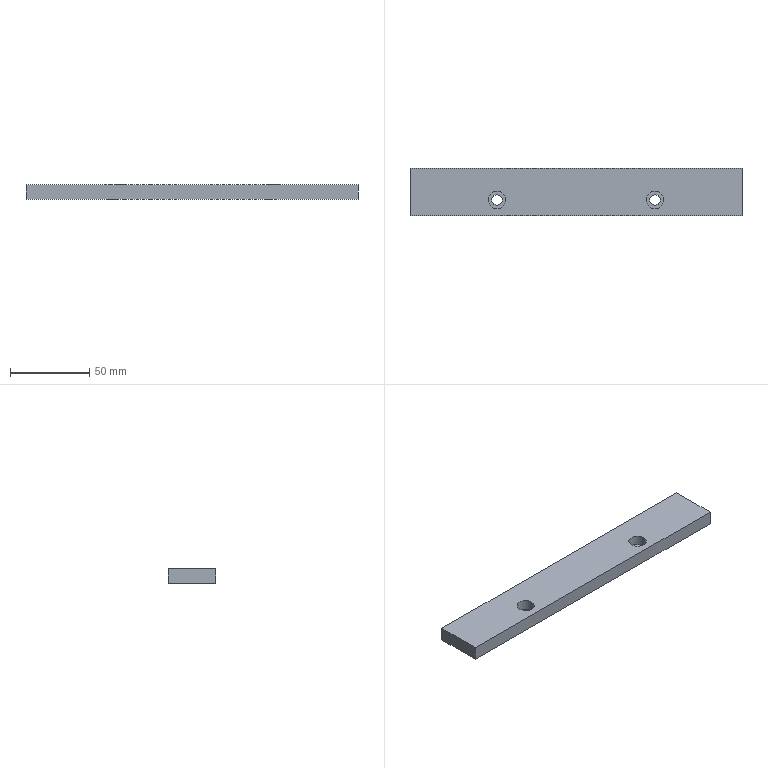Part | STEP file | 0228_209_Stopper | 1 solid | 16 faces | box 210 x 30 x 9 mm | volume 55294 mm3 | cylinder 8 | plane 8 | commonest cylinder face diameters 6.6 x4 11 x4
STEP:
#1=CARTESIAN_POINT('',(0.,0.,0.));
#2=DIRECTION('',(0.,0.,1.));
#3=DIRECTION('',(1.,0.,0.));
#4=AXIS2_PLACEMENT_3D('',#1,#2,#3);
#5=CARTESIAN_POINT('',(-44.5,10.,2.5));
#6=VERTEX_POINT('',#5);
#7=CARTESIAN_POINT('',(-44.5,10.,9.));
#8=VERTEX_POINT('',#7);
#9=CARTESIAN_POINT('',(-44.5,10.,9.));
#10=DIRECTION('',(0.,0.,1.));
#11=VECTOR('',#10,1.);
#12=LINE('',#9,#11);
#13=CARTESIAN_POINT('',(-50.,10.,9.));
#14=DIRECTION('',(0.,0.,1.));
#15=DIRECTION('',(1.,0.,0.));
#16=AXIS2_PLACEMENT_3D('',#13,#14,#15);
#17=CYLINDRICAL_SURFACE('',#16,5.5);
#18=CARTESIAN_POINT('',(6.283,0.));
#19=DIRECTION('',(0.,1.));
#20=VECTOR('',#19,1.);
#21=LINE('',#18,#20);
#22=(GEOMETRIC_REPRESENTATION_CONTEXT(2)PARAMETRIC_REPRESENTATION_CONTEXT()REPRESENTATION_CONTEXT('',''));
#23=DEFINITIONAL_REPRESENTATION('',(#21),#22);
#24=PCURVE('',#17,#23);
#25=CARTESIAN_POINT('',(-50.,10.,9.));
#26=DIRECTION('',(0.,0.,1.));
#27=DIRECTION('',(1.,0.,0.));
#28=AXIS2_PLACEMENT_3D('',#25,#26,#27);
#29=CYLINDRICAL_SURFACE('',#28,5.5);
#30=CARTESIAN_POINT('',(0.,0.));
#31=DIRECTION('',(0.,1.));
#32=VECTOR('',#31,1.);
#33=LINE('',#30,#32);
#34=(GEOMETRIC_REPRESENTATION_CONTEXT(2)PARAMETRIC_REPRESENTATION_CONTEXT()REPRESENTATION_CONTEXT('',''));
#35=DEFINITIONAL_REPRESENTATION('',(#33),#34);
#36=PCURVE('',#29,#35);
#37=SURFACE_CURVE('',#12,(#24,#36),.PCURVE_S1.);
#38=EDGE_CURVE('',#6,#8,#37,.T.);
#39=ORIENTED_EDGE('',*,*,#38,.T.);
#40=CARTESIAN_POINT('',(-55.5,10.,9.));
#41=VERTEX_POINT('',#40);
#42=CARTESIAN_POINT('',(-50.,10.,9.));
#43=DIRECTION('',(0.,0.,1.));
#44=DIRECTION('',(1.,0.,0.));
#45=AXIS2_PLACEMENT_3D('',#42,#43,#44);
#46=CIRCLE('',#45,5.5);
#47=CARTESIAN_POINT('',(0.,0.));
#48=DIRECTION('',(1.,0.));
#49=VECTOR('',#48,1.);
#50=LINE('',#47,#49);
#51=(GEOMETRIC_REPRESENTATION_CONTEXT(2)PARAMETRIC_REPRESENTATION_CONTEXT()REPRESENTATION_CONTEXT('',''));
#52=DEFINITIONAL_REPRESENTATION('',(#50),#51);
#53=PCURVE('',#17,#52);
#54=CARTESIAN_POINT('',(-105.,30.,9.));
#55=DIRECTION('',(0.,0.,-1.));
#56=DIRECTION('',(-1.,0.,0.));
#57=AXIS2_PLACEMENT_3D('',#54,#55,#56);
#58=PLANE('',#57);
#59=CARTESIAN_POINT('',(-60.5,-20.));
#60=CARTESIAN_POINT('',(-60.5,-10.474));
#61=CARTESIAN_POINT('',(-52.25,-15.237));
#62=CARTESIAN_POINT('',(-44.,-20.));
#63=CARTESIAN_POINT('',(-52.25,-24.763));
#64=CARTESIAN_POINT('',(-60.5,-29.526));
#65=CARTESIAN_POINT('',(-60.5,-20.));
#66=(BOUNDED_CURVE()B_SPLINE_CURVE(2,(#59,#60,#61,#62,#63,#64,#65),.UNSPECIFIED.,.T.,.F.)B_SPLINE_CURVE_WITH_KNOTS((1,2,2,2,2,1),(-2.094,0.,2.094,4.189,6.283,8.378),.UNSPECIFIED.)CURVE()GEOMETRIC_REPRESENTATION_ITEM()RATIONAL_B_SPLINE_CURVE((1.,0.5,1.,0.5,1.,0.5,1.))REPRESENTATION_ITEM(''));
#67=(GEOMETRIC_REPRESENTATION_CONTEXT(2)PARAMETRIC_REPRESENTATION_CONTEXT()REPRESENTATION_CONTEXT('',''));
#68=DEFINITIONAL_REPRESENTATION('',(#66),#67);
#69=PCURVE('',#58,#68);
#70=SURFACE_CURVE('',#46,(#53,#69),.PCURVE_S1.);
#71=EDGE_CURVE('',#41,#8,#70,.T.);
#72=ORIENTED_EDGE('',*,*,#71,.F.);
#73=CARTESIAN_POINT('',(-55.5,10.,2.5));
#74=VERTEX_POINT('',#73);
#75=CARTESIAN_POINT('',(-55.5,10.,9.));
#76=DIRECTION('',(0.,0.,1.));
#77=VECTOR('',#76,1.);
#78=LINE('',#75,#77);
#79=CARTESIAN_POINT('',(3.142,0.));
#80=DIRECTION('',(0.,1.));
#81=VECTOR('',#80,1.);
#82=LINE('',#79,#81);
#83=(GEOMETRIC_REPRESENTATION_CONTEXT(2)PARAMETRIC_REPRESENTATION_CONTEXT()REPRESENTATION_CONTEXT('',''));
#84=DEFINITIONAL_REPRESENTATION('',(#82),#83);
#85=PCURVE('',#17,#84);
#86=CARTESIAN_POINT('',(3.142,0.));
#87=DIRECTION('',(0.,1.));
#88=VECTOR('',#87,1.);
#89=LINE('',#86,#88);
#90=(GEOMETRIC_REPRESENTATION_CONTEXT(2)PARAMETRIC_REPRESENTATION_CONTEXT()REPRESENTATION_CONTEXT('',''));
#91=DEFINITIONAL_REPRESENTATION('',(#89),#90);
#92=PCURVE('',#29,#91);
#93=SURFACE_CURVE('',#78,(#85,#92),.PCURVE_S1.);
#94=EDGE_CURVE('',#74,#41,#93,.T.);
#95=ORIENTED_EDGE('',*,*,#94,.F.);
#96=CARTESIAN_POINT('',(-50.,10.,2.5));
#97=DIRECTION('',(0.,0.,1.));
#98=DIRECTION('',(1.,0.,0.));
#99=AXIS2_PLACEMENT_3D('',#96,#97,#98);
#100=CIRCLE('',#99,5.5);
#101=CARTESIAN_POINT('',(0.,-6.5));
#102=DIRECTION('',(1.,0.));
#103=VECTOR('',#102,1.);
#104=LINE('',#101,#103);
#105=(GEOMETRIC_REPRESENTATION_CONTEXT(2)PARAMETRIC_REPRESENTATION_CONTEXT()REPRESENTATION_CONTEXT('',''));
#106=DEFINITIONAL_REPRESENTATION('',(#104),#105);
#107=PCURVE('',#17,#106);
#108=CARTESIAN_POINT('',(-46.7,10.,2.5));
#109=DIRECTION('',(0.,0.,-1.));
#110=DIRECTION('',(-1.,0.,0.));
#111=AXIS2_PLACEMENT_3D('',#108,#109,#110);
#112=PLANE('',#111);
#113=CARTESIAN_POINT('',(-2.2,0.));
#114=CARTESIAN_POINT('',(-2.2,9.526));
#115=CARTESIAN_POINT('',(6.05,4.763));
#116=CARTESIAN_POINT('',(14.3,0.));
#117=CARTESIAN_POINT('',(6.05,-4.763));
#118=CARTESIAN_POINT('',(-2.2,-9.526));
#119=CARTESIAN_POINT('',(-2.2,0.));
#120=(BOUNDED_CURVE()B_SPLINE_CURVE(2,(#113,#114,#115,#116,#117,#118,#119),.UNSPECIFIED.,.T.,.F.)B_SPLINE_CURVE_WITH_KNOTS((1,2,2,2,2,1),(-2.094,0.,2.094,4.189,6.283,8.378),.UNSPECIFIED.)CURVE()GEOMETRIC_REPRESENTATION_ITEM()RATIONAL_B_SPLINE_CURVE((1.,0.5,1.,0.5,1.,0.5,1.))REPRESENTATION_ITEM(''));
#121=(GEOMETRIC_REPRESENTATION_CONTEXT(2)PARAMETRIC_REPRESENTATION_CONTEXT()REPRESENTATION_CONTEXT('',''));
#122=DEFINITIONAL_REPRESENTATION('',(#120),#121);
#123=PCURVE('',#112,#122);
#124=SURFACE_CURVE('',#100,(#107,#123),.PCURVE_S1.);
#125=EDGE_CURVE('',#74,#6,#124,.T.);
#126=ORIENTED_EDGE('',*,*,#125,.T.);
#127=EDGE_LOOP('',(#39,#72,#95,#126));
#128=FACE_BOUND('',#127,.F.);
#129=ADVANCED_FACE('',(#128),#17,.F.);
#130=CARTESIAN_POINT('',(-46.7,10.,0.));
#131=VERTEX_POINT('',#130);
#132=CARTESIAN_POINT('',(-46.7,10.,2.5));
#133=VERTEX_POINT('',#132);
#134=CARTESIAN_POINT('',(-46.7,10.,9.));
#135=DIRECTION('',(0.,0.,1.));
#136=VECTOR('',#135,1.);
#137=LINE('',#134,#136);
#138=CARTESIAN_POINT('',(-50.,10.,9.));
#139=DIRECTION('',(0.,0.,1.));
#140=DIRECTION('',(1.,0.,0.));
#141=AXIS2_PLACEMENT_3D('',#138,#139,#140);
#142=CYLINDRICAL_SURFACE('',#141,3.3);
#143=CARTESIAN_POINT('',(6.283,0.));
#144=DIRECTION('',(0.,1.));
#145=VECTOR('',#144,1.);
#146=LINE('',#143,#145);
#147=(GEOMETRIC_REPRESENTATION_CONTEXT(2)PARAMETRIC_REPRESENTATION_CONTEXT()REPRESENTATION_CONTEXT('',''));
#148=DEFINITIONAL_REPRESENTATION('',(#146),#147);
#149=PCURVE('',#142,#148);
#150=CARTESIAN_POINT('',(-50.,10.,9.));
#151=DIRECTION('',(0.,0.,1.));
#152=DIRECTION('',(1.,0.,0.));
#153=AXIS2_PLACEMENT_3D('',#150,#151,#152);
#154=CYLINDRICAL_SURFACE('',#153,3.3);
#155=CARTESIAN_POINT('',(0.,0.));
#156=DIRECTION('',(0.,1.));
#157=VECTOR('',#156,1.);
#158=LINE('',#155,#157);
#159=(GEOMETRIC_REPRESENTATION_CONTEXT(2)PARAMETRIC_REPRESENTATION_CONTEXT()REPRESENTATION_CONTEXT('',''));
#160=DEFINITIONAL_REPRESENTATION('',(#158),#159);
#161=PCURVE('',#154,#160);
#162=SURFACE_CURVE('',#137,(#149,#161),.PCURVE_S1.);
#163=EDGE_CURVE('',#131,#133,#162,.T.);
#164=ORIENTED_EDGE('',*,*,#163,.T.);
#165=CARTESIAN_POINT('',(-53.3,10.,2.5));
#166=VERTEX_POINT('',#165);
#167=CARTESIAN_POINT('',(-50.,10.,2.5));
#168=DIRECTION('',(0.,0.,1.));
#169=DIRECTION('',(1.,0.,0.));
#170=AXIS2_PLACEMENT_3D('',#167,#168,#169);
#171=CIRCLE('',#170,3.3);
#172=CARTESIAN_POINT('',(0.,-6.5));
#173=DIRECTION('',(1.,0.));
#174=VECTOR('',#173,1.);
#175=LINE('',#172,#174);
#176=(GEOMETRIC_REPRESENTATION_CONTEXT(2)PARAMETRIC_REPRESENTATION_CONTEXT()REPRESENTATION_CONTEXT('',''));
#177=DEFINITIONAL_REPRESENTATION('',(#175),#176);
#178=PCURVE('',#142,#177);
#179=CARTESIAN_POINT('',(0.,0.));
#180=CARTESIAN_POINT('',(0.,5.716));
#181=CARTESIAN_POINT('',(4.95,2.858));
#182=CARTESIAN_POINT('',(9.9,0.));
#183=CARTESIAN_POINT('',(4.95,-2.858));
#184=CARTESIAN_POINT('',(0.,-5.716));
#185=CARTESIAN_POINT('',(0.,0.));
#186=(BOUNDED_CURVE()B_SPLINE_CURVE(2,(#179,#180,#181,#182,#183,#184,#185),.UNSPECIFIED.,.T.,.F.)B_SPLINE_CURVE_WITH_KNOTS((1,2,2,2,2,1),(-2.094,0.,2.094,4.189,6.283,8.378),.UNSPECIFIED.)CURVE()GEOMETRIC_REPRESENTATION_ITEM()RATIONAL_B_SPLINE_CURVE((1.,0.5,1.,0.5,1.,0.5,1.))REPRESENTATION_ITEM(''));
#187=(GEOMETRIC_REPRESENTATION_CONTEXT(2)PARAMETRIC_REPRESENTATION_CONTEXT()REPRESENTATION_CONTEXT('',''));
#188=DEFINITIONAL_REPRESENTATION('',(#186),#187);
#189=PCURVE('',#112,#188);
#190=SURFACE_CURVE('',#171,(#178,#189),.PCURVE_S1.);
#191=EDGE_CURVE('',#166,#133,#190,.T.);
#192=ORIENTED_EDGE('',*,*,#191,.F.);
#193=CARTESIAN_POINT('',(-53.3,10.,0.));
#194=VERTEX_POINT('',#193);
#195=CARTESIAN_POINT('',(-53.3,10.,9.));
#196=DIRECTION('',(0.,0.,1.));
#197=VECTOR('',#196,1.);
#198=LINE('',#195,#197);
#199=CARTESIAN_POINT('',(3.142,0.));
#200=DIRECTION('',(0.,1.));
#201=VECTOR('',#200,1.);
#202=LINE('',#199,#201);
#203=(GEOMETRIC_REPRESENTATION_CONTEXT(2)PARAMETRIC_REPRESENTATION_CONTEXT()REPRESENTATION_CONTEXT('',''));
#204=DEFINITIONAL_REPRESENTATION('',(#202),#203);
#205=PCURVE('',#142,#204);
#206=CARTESIAN_POINT('',(3.142,0.));
#207=DIRECTION('',(0.,1.));
#208=VECTOR('',#207,1.);
#209=LINE('',#206,#208);
#210=(GEOMETRIC_REPRESENTATION_CONTEXT(2)PARAMETRIC_REPRESENTATION_CONTEXT()REPRESENTATION_CONTEXT('',''));
#211=DEFINITIONAL_REPRESENTATION('',(#209),#210);
#212=PCURVE('',#154,#211);
#213=SURFACE_CURVE('',#198,(#205,#212),.PCURVE_S1.);
#214=EDGE_CURVE('',#194,#166,#213,.T.);
#215=ORIENTED_EDGE('',*,*,#214,.F.);
#216=CARTESIAN_POINT('',(-50.,10.,0.));
#217=DIRECTION('',(0.,0.,1.));
#218=DIRECTION('',(1.,0.,0.));
#219=AXIS2_PLACEMENT_3D('',#216,#217,#218);
#220=CIRCLE('',#219,3.3);
#221=CARTESIAN_POINT('',(0.,-9.));
#222=DIRECTION('',(1.,0.));
#223=VECTOR('',#222,1.);
#224=LINE('',#221,#223);
#225=(GEOMETRIC_REPRESENTATION_CONTEXT(2)PARAMETRIC_REPRESENTATION_CONTEXT()REPRESENTATION_CONTEXT('',''));
#226=DEFINITIONAL_REPRESENTATION('',(#224),#225);
#227=PCURVE('',#142,#226);
#228=CARTESIAN_POINT('',(-105.,30.,0.));
#229=DIRECTION('',(0.,0.,-1.));
#230=DIRECTION('',(-1.,0.,0.));
#231=AXIS2_PLACEMENT_3D('',#228,#229,#230);
#232=PLANE('',#231);
#233=CARTESIAN_POINT('',(-58.3,-20.));
#234=CARTESIAN_POINT('',(-58.3,-14.284));
#235=CARTESIAN_POINT('',(-53.35,-17.142));
#236=CARTESIAN_POINT('',(-48.4,-20.));
#237=CARTESIAN_POINT('',(-53.35,-22.858));
#238=CARTESIAN_POINT('',(-58.3,-25.716));
#239=CARTESIAN_POINT('',(-58.3,-20.));
#240=(BOUNDED_CURVE()B_SPLINE_CURVE(2,(#233,#234,#235,#236,#237,#238,#239),.UNSPECIFIED.,.T.,.F.)B_SPLINE_CURVE_WITH_KNOTS((1,2,2,2,2,1),(-2.094,0.,2.094,4.189,6.283,8.378),.UNSPECIFIED.)CURVE()GEOMETRIC_REPRESENTATION_ITEM()RATIONAL_B_SPLINE_CURVE((1.,0.5,1.,0.5,1.,0.5,1.))REPRESENTATION_ITEM(''));
#241=(GEOMETRIC_REPRESENTATION_CONTEXT(2)PARAMETRIC_REPRESENTATION_CONTEXT()REPRESENTATION_CONTEXT('',''));
#242=DEFINITIONAL_REPRESENTATION('',(#240),#241);
#243=PCURVE('',#232,#242);
#244=SURFACE_CURVE('',#220,(#227,#243),.PCURVE_S1.);
#245=EDGE_CURVE('',#194,#131,#244,.T.);
#246=ORIENTED_EDGE('',*,*,#245,.T.);
#247=EDGE_LOOP('',(#164,#192,#215,#246));
#248=FACE_BOUND('',#247,.F.);
#249=ADVANCED_FACE('',(#248),#142,.F.);
#250=CARTESIAN_POINT('',(55.5,10.,2.5));
#251=VERTEX_POINT('',#250);
#252=CARTESIAN_POINT('',(55.5,10.,9.));
#253=VERTEX_POINT('',#252);
#254=CARTESIAN_POINT('',(55.5,10.,9.));
#255=DIRECTION('',(0.,0.,1.));
#256=VECTOR('',#255,1.);
#257=LINE('',#254,#256);
#258=CARTESIAN_POINT('',(50.,10.,9.));
#259=DIRECTION('',(0.,0.,1.));
#260=DIRECTION('',(1.,0.,0.));
#261=AXIS2_PLACEMENT_3D('',#258,#259,#260);
#262=CYLINDRICAL_SURFACE('',#261,5.5);
#263=CARTESIAN_POINT('',(6.283,0.));
#264=DIRECTION('',(0.,1.));
#265=VECTOR('',#264,1.);
#266=LINE('',#263,#265);
#267=(GEOMETRIC_REPRESENTATION_CONTEXT(2)PARAMETRIC_REPRESENTATION_CONTEXT()REPRESENTATION_CONTEXT('',''));
#268=DEFINITIONAL_REPRESENTATION('',(#266),#267);
#269=PCURVE('',#262,#268);
#270=CARTESIAN_POINT('',(50.,10.,9.));
#271=DIRECTION('',(0.,0.,1.));
#272=DIRECTION('',(1.,0.,0.));
#273=AXIS2_PLACEMENT_3D('',#270,#271,#272);
#274=CYLINDRICAL_SURFACE('',#273,5.5);
#275=CARTESIAN_POINT('',(0.,0.));
#276=DIRECTION('',(0.,1.));
#277=VECTOR('',#276,1.);
#278=LINE('',#275,#277);
#279=(GEOMETRIC_REPRESENTATION_CONTEXT(2)PARAMETRIC_REPRESENTATION_CONTEXT()REPRESENTATION_CONTEXT('',''));
#280=DEFINITIONAL_REPRESENTATION('',(#278),#279);
#281=PCURVE('',#274,#280);
#282=SURFACE_CURVE('',#257,(#269,#281),.PCURVE_S1.);
#283=EDGE_CURVE('',#251,#253,#282,.T.);
#284=ORIENTED_EDGE('',*,*,#283,.T.);
#285=CARTESIAN_POINT('',(44.5,10.,9.));
#286=VERTEX_POINT('',#285);
#287=CARTESIAN_POINT('',(50.,10.,9.));
#288=DIRECTION('',(0.,0.,1.));
#289=DIRECTION('',(1.,0.,0.));
#290=AXIS2_PLACEMENT_3D('',#287,#288,#289);
#291=CIRCLE('',#290,5.5);
#292=CARTESIAN_POINT('',(0.,0.));
#293=DIRECTION('',(1.,0.));
#294=VECTOR('',#293,1.);
#295=LINE('',#292,#294);
#296=(GEOMETRIC_REPRESENTATION_CONTEXT(2)PARAMETRIC_REPRESENTATION_CONTEXT()REPRESENTATION_CONTEXT('',''));
#297=DEFINITIONAL_REPRESENTATION('',(#295),#296);
#298=PCURVE('',#262,#297);
#299=CARTESIAN_POINT('',(-160.5,-20.));
#300=CARTESIAN_POINT('',(-160.5,-10.474));
#301=CARTESIAN_POINT('',(-152.25,-15.237));
#302=CARTESIAN_POINT('',(-144.,-20.));
#303=CARTESIAN_POINT('',(-152.25,-24.763));
#304=CARTESIAN_POINT('',(-160.5,-29.526));
#305=CARTESIAN_POINT('',(-160.5,-20.));
#306=(BOUNDED_CURVE()B_SPLINE_CURVE(2,(#299,#300,#301,#302,#303,#304,#305),.UNSPECIFIED.,.T.,.F.)B_SPLINE_CURVE_WITH_KNOTS((1,2,2,2,2,1),(-2.094,0.,2.094,4.189,6.283,8.378),.UNSPECIFIED.)CURVE()GEOMETRIC_REPRESENTATION_ITEM()RATIONAL_B_SPLINE_CURVE((1.,0.5,1.,0.5,1.,0.5,1.))REPRESENTATION_ITEM(''));
#307=(GEOMETRIC_REPRESENTATION_CONTEXT(2)PARAMETRIC_REPRESENTATION_CONTEXT()REPRESENTATION_CONTEXT('',''));
#308=DEFINITIONAL_REPRESENTATION('',(#306),#307);
#309=PCURVE('',#58,#308);
#310=SURFACE_CURVE('',#291,(#298,#309),.PCURVE_S1.);
#311=EDGE_CURVE('',#286,#253,#310,.T.);
#312=ORIENTED_EDGE('',*,*,#311,.F.);
#313=CARTESIAN_POINT('',(44.5,10.,2.5));
#314=VERTEX_POINT('',#313);
#315=CARTESIAN_POINT('',(44.5,10.,9.));
#316=DIRECTION('',(0.,0.,1.));
#317=VECTOR('',#316,1.);
#318=LINE('',#315,#317);
#319=CARTESIAN_POINT('',(3.142,0.));
#320=DIRECTION('',(0.,1.));
#321=VECTOR('',#320,1.);
#322=LINE('',#319,#321);
#323=(GEOMETRIC_REPRESENTATION_CONTEXT(2)PARAMETRIC_REPRESENTATION_CONTEXT()REPRESENTATION_CONTEXT('',''));
#324=DEFINITIONAL_REPRESENTATION('',(#322),#323);
#325=PCURVE('',#262,#324);
#326=CARTESIAN_POINT('',(3.142,0.));
#327=DIRECTION('',(0.,1.));
#328=VECTOR('',#327,1.);
#329=LINE('',#326,#328);
#330=(GEOMETRIC_REPRESENTATION_CONTEXT(2)PARAMETRIC_REPRESENTATION_CONTEXT()REPRESENTATION_CONTEXT('',''));
#331=DEFINITIONAL_REPRESENTATION('',(#329),#330);
#332=PCURVE('',#274,#331);
#333=SURFACE_CURVE('',#318,(#325,#332),.PCURVE_S1.);
#334=EDGE_CURVE('',#314,#286,#333,.T.);
#335=ORIENTED_EDGE('',*,*,#334,.F.);
#336=CARTESIAN_POINT('',(50.,10.,2.5));
#337=DIRECTION('',(0.,0.,1.));
#338=DIRECTION('',(1.,0.,0.));
#339=AXIS2_PLACEMENT_3D('',#336,#337,#338);
#340=CIRCLE('',#339,5.5);
#341=CARTESIAN_POINT('',(0.,-6.5));
#342=DIRECTION('',(1.,0.));
#343=VECTOR('',#342,1.);
#344=LINE('',#341,#343);
#345=(GEOMETRIC_REPRESENTATION_CONTEXT(2)PARAMETRIC_REPRESENTATION_CONTEXT()REPRESENTATION_CONTEXT('',''));
#346=DEFINITIONAL_REPRESENTATION('',(#344),#345);
#347=PCURVE('',#262,#346);
#348=CARTESIAN_POINT('',(53.3,10.,2.5));
#349=DIRECTION('',(0.,0.,-1.));
#350=DIRECTION('',(-1.,0.,0.));
#351=AXIS2_PLACEMENT_3D('',#348,#349,#350);
#352=PLANE('',#351);
#353=CARTESIAN_POINT('',(-2.2,0.));
#354=CARTESIAN_POINT('',(-2.2,9.526));
#355=CARTESIAN_POINT('',(6.05,4.763));
#356=CARTESIAN_POINT('',(14.3,0.));
#357=CARTESIAN_POINT('',(6.05,-4.763));
#358=CARTESIAN_POINT('',(-2.2,-9.526));
#359=CARTESIAN_POINT('',(-2.2,0.));
#360=(BOUNDED_CURVE()B_SPLINE_CURVE(2,(#353,#354,#355,#356,#357,#358,#359),.UNSPECIFIED.,.T.,.F.)B_SPLINE_CURVE_WITH_KNOTS((1,2,2,2,2,1),(-2.094,0.,2.094,4.189,6.283,8.378),.UNSPECIFIED.)CURVE()GEOMETRIC_REPRESENTATION_ITEM()RATIONAL_B_SPLINE_CURVE((1.,0.5,1.,0.5,1.,0.5,1.))REPRESENTATION_ITEM(''));
#361=(GEOMETRIC_REPRESENTATION_CONTEXT(2)PARAMETRIC_REPRESENTATION_CONTEXT()REPRESENTATION_CONTEXT('',''));
#362=DEFINITIONAL_REPRESENTATION('',(#360),#361);
#363=PCURVE('',#352,#362);
#364=SURFACE_CURVE('',#340,(#347,#363),.PCURVE_S1.);
#365=EDGE_CURVE('',#314,#251,#364,.T.);
#366=ORIENTED_EDGE('',*,*,#365,.T.);
#367=EDGE_LOOP('',(#284,#312,#335,#366));
#368=FACE_BOUND('',#367,.F.);
#369=ADVANCED_FACE('',(#368),#262,.F.);
#370=CARTESIAN_POINT('',(53.3,10.,0.));
#371=VERTEX_POINT('',#370);
#372=CARTESIAN_POINT('',(53.3,10.,2.5));
#373=VERTEX_POINT('',#372);
#374=CARTESIAN_POINT('',(53.3,10.,9.));
#375=DIRECTION('',(0.,0.,1.));
#376=VECTOR('',#375,1.);
#377=LINE('',#374,#376);
#378=CARTESIAN_POINT('',(50.,10.,9.));
#379=DIRECTION('',(0.,0.,1.));
#380=DIRECTION('',(1.,0.,0.));
#381=AXIS2_PLACEMENT_3D('',#378,#379,#380);
#382=CYLINDRICAL_SURFACE('',#381,3.3);
#383=CARTESIAN_POINT('',(6.283,0.));
#384=DIRECTION('',(0.,1.));
#385=VECTOR('',#384,1.);
#386=LINE('',#383,#385);
#387=(GEOMETRIC_REPRESENTATION_CONTEXT(2)PARAMETRIC_REPRESENTATION_CONTEXT()REPRESENTATION_CONTEXT('',''));
#388=DEFINITIONAL_REPRESENTATION('',(#386),#387);
#389=PCURVE('',#382,#388);
#390=CARTESIAN_POINT('',(50.,10.,9.));
#391=DIRECTION('',(0.,0.,1.));
#392=DIRECTION('',(1.,0.,0.));
#393=AXIS2_PLACEMENT_3D('',#390,#391,#392);
#394=CYLINDRICAL_SURFACE('',#393,3.3);
#395=CARTESIAN_POINT('',(0.,0.));
#396=DIRECTION('',(0.,1.));
#397=VECTOR('',#396,1.);
#398=LINE('',#395,#397);
#399=(GEOMETRIC_REPRESENTATION_CONTEXT(2)PARAMETRIC_REPRESENTATION_CONTEXT()REPRESENTATION_CONTEXT('',''));
#400=DEFINITIONAL_REPRESENTATION('',(#398),#399);
#401=PCURVE('',#394,#400);
#402=SURFACE_CURVE('',#377,(#389,#401),.PCURVE_S1.);
#403=EDGE_CURVE('',#371,#373,#402,.T.);
#404=ORIENTED_EDGE('',*,*,#403,.T.);
#405=CARTESIAN_POINT('',(46.7,10.,2.5));
#406=VERTEX_POINT('',#405);
#407=CARTESIAN_POINT('',(50.,10.,2.5));
#408=DIRECTION('',(0.,0.,1.));
#409=DIRECTION('',(1.,0.,0.));
#410=AXIS2_PLACEMENT_3D('',#407,#408,#409);
#411=CIRCLE('',#410,3.3);
#412=CARTESIAN_POINT('',(0.,-6.5));
#413=DIRECTION('',(1.,0.));
#414=VECTOR('',#413,1.);
#415=LINE('',#412,#414);
#416=(GEOMETRIC_REPRESENTATION_CONTEXT(2)PARAMETRIC_REPRESENTATION_CONTEXT()REPRESENTATION_CONTEXT('',''));
#417=DEFINITIONAL_REPRESENTATION('',(#415),#416);
#418=PCURVE('',#382,#417);
#419=CARTESIAN_POINT('',(0.,0.));
#420=CARTESIAN_POINT('',(0.,5.716));
#421=CARTESIAN_POINT('',(4.95,2.858));
#422=CARTESIAN_POINT('',(9.9,0.));
#423=CARTESIAN_POINT('',(4.95,-2.858));
#424=CARTESIAN_POINT('',(0.,-5.716));
#425=CARTESIAN_POINT('',(0.,0.));
#426=(BOUNDED_CURVE()B_SPLINE_CURVE(2,(#419,#420,#421,#422,#423,#424,#425),.UNSPECIFIED.,.T.,.F.)B_SPLINE_CURVE_WITH_KNOTS((1,2,2,2,2,1),(-2.094,0.,2.094,4.189,6.283,8.378),.UNSPECIFIED.)CURVE()GEOMETRIC_REPRESENTATION_ITEM()RATIONAL_B_SPLINE_CURVE((1.,0.5,1.,0.5,1.,0.5,1.))REPRESENTATION_ITEM(''));
#427=(GEOMETRIC_REPRESENTATION_CONTEXT(2)PARAMETRIC_REPRESENTATION_CONTEXT()REPRESENTATION_CONTEXT('',''));
#428=DEFINITIONAL_REPRESENTATION('',(#426),#427);
#429=PCURVE('',#352,#428);
#430=SURFACE_CURVE('',#411,(#418,#429),.PCURVE_S1.);
#431=EDGE_CURVE('',#406,#373,#430,.T.);
#432=ORIENTED_EDGE('',*,*,#431,.F.);
#433=CARTESIAN_POINT('',(46.7,10.,0.));
#434=VERTEX_POINT('',#433);
#435=CARTESIAN_POINT('',(46.7,10.,9.));
#436=DIRECTION('',(0.,0.,1.));
#437=VECTOR('',#436,1.);
#438=LINE('',#435,#437);
#439=CARTESIAN_POINT('',(3.142,0.));
#440=DIRECTION('',(0.,1.));
#441=VECTOR('',#440,1.);
#442=LINE('',#439,#441);
#443=(GEOMETRIC_REPRESENTATION_CONTEXT(2)PARAMETRIC_REPRESENTATION_CONTEXT()REPRESENTATION_CONTEXT('',''));
#444=DEFINITIONAL_REPRESENTATION('',(#442),#443);
#445=PCURVE('',#382,#444);
#446=CARTESIAN_POINT('',(3.142,0.));
#447=DIRECTION('',(0.,1.));
#448=VECTOR('',#447,1.);
#449=LINE('',#446,#448);
#450=(GEOMETRIC_REPRESENTATION_CONTEXT(2)PARAMETRIC_REPRESENTATION_CONTEXT()REPRESENTATION_CONTEXT('',''));
#451=DEFINITIONAL_REPRESENTATION('',(#449),#450);
#452=PCURVE('',#394,#451);
#453=SURFACE_CURVE('',#438,(#445,#452),.PCURVE_S1.);
#454=EDGE_CURVE('',#434,#406,#453,.T.);
#455=ORIENTED_EDGE('',*,*,#454,.F.);
#456=CARTESIAN_POINT('',(50.,10.,0.));
#457=DIRECTION('',(0.,0.,1.));
#458=DIRECTION('',(1.,0.,0.));
#459=AXIS2_PLACEMENT_3D('',#456,#457,#458);
#460=CIRCLE('',#459,3.3);
#461=CARTESIAN_POINT('',(0.,-9.));
#462=DIRECTION('',(1.,0.));
#463=VECTOR('',#462,1.);
#464=LINE('',#461,#463);
#465=(GEOMETRIC_REPRESENTATION_CONTEXT(2)PARAMETRIC_REPRESENTATION_CONTEXT()REPRESENTATION_CONTEXT('',''));
#466=DEFINITIONAL_REPRESENTATION('',(#464),#465);
#467=PCURVE('',#382,#466);
#468=CARTESIAN_POINT('',(-158.3,-20.));
#469=CARTESIAN_POINT('',(-158.3,-14.284));
#470=CARTESIAN_POINT('',(-153.35,-17.142));
#471=CARTESIAN_POINT('',(-148.4,-20.));
#472=CARTESIAN_POINT('',(-153.35,-22.858));
#473=CARTESIAN_POINT('',(-158.3,-25.716));
#474=CARTESIAN_POINT('',(-158.3,-20.));
#475=(BOUNDED_CURVE()B_SPLINE_CURVE(2,(#468,#469,#470,#471,#472,#473,#474),.UNSPECIFIED.,.T.,.F.)B_SPLINE_CURVE_WITH_KNOTS((1,2,2,2,2,1),(-2.094,0.,2.094,4.189,6.283,8.378),.UNSPECIFIED.)CURVE()GEOMETRIC_REPRESENTATION_ITEM()RATIONAL_B_SPLINE_CURVE((1.,0.5,1.,0.5,1.,0.5,1.))REPRESENTATION_ITEM(''));
#476=(GEOMETRIC_REPRESENTATION_CONTEXT(2)PARAMETRIC_REPRESENTATION_CONTEXT()REPRESENTATION_CONTEXT('',''));
#477=DEFINITIONAL_REPRESENTATION('',(#475),#476);
#478=PCURVE('',#232,#477);
#479=SURFACE_CURVE('',#460,(#467,#478),.PCURVE_S1.);
#480=EDGE_CURVE('',#434,#371,#479,.T.);
#481=ORIENTED_EDGE('',*,*,#480,.T.);
#482=EDGE_LOOP('',(#404,#432,#455,#481));
#483=FACE_BOUND('',#482,.F.);
#484=ADVANCED_FACE('',(#483),#382,.F.);
#485=CARTESIAN_POINT('',(-105.,30.,0.));
#486=VERTEX_POINT('',#485);
#487=CARTESIAN_POINT('',(-105.,0.,0.));
#488=VERTEX_POINT('',#487);
#489=CARTESIAN_POINT('',(-105.,0.,0.));
#490=DIRECTION('',(0.,-1.,0.));
#491=VECTOR('',#490,1.);
#492=LINE('',#489,#491);
#493=CARTESIAN_POINT('',(-105.,0.,9.));
#494=DIRECTION('',(1.,0.,0.));
#495=DIRECTION('',(0.,0.,-1.));
#496=AXIS2_PLACEMENT_3D('',#493,#494,#495);
#497=PLANE('',#496);
#498=CARTESIAN_POINT('',(9.,0.));
#499=DIRECTION('',(0.,-1.));
#500=VECTOR('',#499,1.);
#501=LINE('',#498,#500);
#502=(GEOMETRIC_REPRESENTATION_CONTEXT(2)PARAMETRIC_REPRESENTATION_CONTEXT()REPRESENTATION_CONTEXT('',''));
#503=DEFINITIONAL_REPRESENTATION('',(#501),#502);
#504=PCURVE('',#497,#503);
#505=CARTESIAN_POINT('',(0.,-30.));
#506=DIRECTION('',(0.,-1.));
#507=VECTOR('',#506,1.);
#508=LINE('',#505,#507);
#509=(GEOMETRIC_REPRESENTATION_CONTEXT(2)PARAMETRIC_REPRESENTATION_CONTEXT()REPRESENTATION_CONTEXT('',''));
#510=DEFINITIONAL_REPRESENTATION('',(#508),#509);
#511=PCURVE('',#232,#510);
#512=SURFACE_CURVE('',#492,(#504,#511),.PCURVE_S1.);
#513=EDGE_CURVE('',#486,#488,#512,.T.);
#514=ORIENTED_EDGE('',*,*,#513,.T.);
#515=CARTESIAN_POINT('',(-105.,0.,9.));
#516=VERTEX_POINT('',#515);
#517=CARTESIAN_POINT('',(-105.,0.,9.));
#518=DIRECTION('',(0.,0.,-1.));
#519=VECTOR('',#518,1.);
#520=LINE('',#517,#519);
#521=CARTESIAN_POINT('',(0.,0.));
#522=DIRECTION('',(1.,0.));
#523=VECTOR('',#522,1.);
#524=LINE('',#521,#523);
#525=(GEOMETRIC_REPRESENTATION_CONTEXT(2)PARAMETRIC_REPRESENTATION_CONTEXT()REPRESENTATION_CONTEXT('',''));
#526=DEFINITIONAL_REPRESENTATION('',(#524),#525);
#527=PCURVE('',#497,#526);
#528=CARTESIAN_POINT('',(-105.,0.,9.));
#529=DIRECTION('',(0.,1.,0.));
#530=DIRECTION('',(0.,0.,1.));
#531=AXIS2_PLACEMENT_3D('',#528,#529,#530);
#532=PLANE('',#531);
#533=CARTESIAN_POINT('',(0.,0.));
#534=DIRECTION('',(-1.,0.));
#535=VECTOR('',#534,1.);
#536=LINE('',#533,#535);
#537=(GEOMETRIC_REPRESENTATION_CONTEXT(2)PARAMETRIC_REPRESENTATION_CONTEXT()REPRESENTATION_CONTEXT('',''));
#538=DEFINITIONAL_REPRESENTATION('',(#536),#537);
#539=PCURVE('',#532,#538);
#540=SURFACE_CURVE('',#520,(#527,#539),.PCURVE_S1.);
#541=EDGE_CURVE('',#516,#488,#540,.T.);
#542=ORIENTED_EDGE('',*,*,#541,.F.);
#543=CARTESIAN_POINT('',(-105.,30.,9.));
#544=VERTEX_POINT('',#543);
#545=CARTESIAN_POINT('',(-105.,0.,9.));
#546=DIRECTION('',(0.,-1.,0.));
#547=VECTOR('',#546,1.);
#548=LINE('',#545,#547);
#549=CARTESIAN_POINT('',(0.,0.));
#550=DIRECTION('',(0.,-1.));
#551=VECTOR('',#550,1.);
#552=LINE('',#549,#551);
#553=(GEOMETRIC_REPRESENTATION_CONTEXT(2)PARAMETRIC_REPRESENTATION_CONTEXT()REPRESENTATION_CONTEXT('',''));
#554=DEFINITIONAL_REPRESENTATION('',(#552),#553);
#555=PCURVE('',#497,#554);
#556=CARTESIAN_POINT('',(0.,-30.));
#557=DIRECTION('',(0.,-1.));
#558=VECTOR('',#557,1.);
#559=LINE('',#556,#558);
#560=(GEOMETRIC_REPRESENTATION_CONTEXT(2)PARAMETRIC_REPRESENTATION_CONTEXT()REPRESENTATION_CONTEXT('',''));
#561=DEFINITIONAL_REPRESENTATION('',(#559),#560);
#562=PCURVE('',#58,#561);
#563=SURFACE_CURVE('',#548,(#555,#562),.PCURVE_S1.);
#564=EDGE_CURVE('',#544,#516,#563,.T.);
#565=ORIENTED_EDGE('',*,*,#564,.F.);
#566=CARTESIAN_POINT('',(-105.,30.,9.));
#567=DIRECTION('',(0.,0.,-1.));
#568=VECTOR('',#567,1.);
#569=LINE('',#566,#568);
#570=CARTESIAN_POINT('',(0.,30.));
#571=DIRECTION('',(1.,0.));
#572=VECTOR('',#571,1.);
#573=LINE('',#570,#572);
#574=(GEOMETRIC_REPRESENTATION_CONTEXT(2)PARAMETRIC_REPRESENTATION_CONTEXT()REPRESENTATION_CONTEXT('',''));
#575=DEFINITIONAL_REPRESENTATION('',(#573),#574);
#576=PCURVE('',#497,#575);
#577=CARTESIAN_POINT('',(-105.,30.,9.));
#578=DIRECTION('',(0.,-1.,0.));
#579=DIRECTION('',(0.,0.,-1.));
#580=AXIS2_PLACEMENT_3D('',#577,#578,#579);
#581=PLANE('',#580);
#582=CARTESIAN_POINT('',(0.,0.));
#583=DIRECTION('',(1.,0.));
#584=VECTOR('',#583,1.);
#585=LINE('',#582,#584);
#586=(GEOMETRIC_REPRESENTATION_CONTEXT(2)PARAMETRIC_REPRESENTATION_CONTEXT()REPRESENTATION_CONTEXT('',''));
#587=DEFINITIONAL_REPRESENTATION('',(#585),#586);
#588=PCURVE('',#581,#587);
#589=SURFACE_CURVE('',#569,(#576,#588),.PCURVE_S1.);
#590=EDGE_CURVE('',#544,#486,#589,.T.);
#591=ORIENTED_EDGE('',*,*,#590,.T.);
#592=EDGE_LOOP('',(#514,#542,#565,#591));
#593=FACE_BOUND('',#592,.T.);
#594=ADVANCED_FACE('',(#593),#497,.F.);
#595=CARTESIAN_POINT('',(105.,0.,0.));
#596=VERTEX_POINT('',#595);
#597=CARTESIAN_POINT('',(-105.,0.,0.));
#598=DIRECTION('',(1.,0.,0.));
#599=VECTOR('',#598,1.);
#600=LINE('',#597,#599);
#601=CARTESIAN_POINT('',(-9.,0.));
#602=DIRECTION('',(0.,1.));
#603=VECTOR('',#602,1.);
#604=LINE('',#601,#603);
#605=(GEOMETRIC_REPRESENTATION_CONTEXT(2)PARAMETRIC_REPRESENTATION_CONTEXT()REPRESENTATION_CONTEXT('',''));
#606=DEFINITIONAL_REPRESENTATION('',(#604),#605);
#607=PCURVE('',#532,#606);
#608=CARTESIAN_POINT('',(0.,-30.));
#609=DIRECTION('',(-1.,0.));
#610=VECTOR('',#609,1.);
#611=LINE('',#608,#610);
#612=(GEOMETRIC_REPRESENTATION_CONTEXT(2)PARAMETRIC_REPRESENTATION_CONTEXT()REPRESENTATION_CONTEXT('',''));
#613=DEFINITIONAL_REPRESENTATION('',(#611),#612);
#614=PCURVE('',#232,#613);
#615=SURFACE_CURVE('',#600,(#607,#614),.PCURVE_S1.);
#616=EDGE_CURVE('',#488,#596,#615,.T.);
#617=ORIENTED_EDGE('',*,*,#616,.T.);
#618=CARTESIAN_POINT('',(105.,0.,9.));
#619=VERTEX_POINT('',#618);
#620=CARTESIAN_POINT('',(105.,0.,9.));
#621=DIRECTION('',(0.,0.,-1.));
#622=VECTOR('',#621,1.);
#623=LINE('',#620,#622);
#624=CARTESIAN_POINT('',(0.,210.));
#625=DIRECTION('',(-1.,0.));
#626=VECTOR('',#625,1.);
#627=LINE('',#624,#626);
#628=(GEOMETRIC_REPRESENTATION_CONTEXT(2)PARAMETRIC_REPRESENTATION_CONTEXT()REPRESENTATION_CONTEXT('',''));
#629=DEFINITIONAL_REPRESENTATION('',(#627),#628);
#630=PCURVE('',#532,#629);
#631=CARTESIAN_POINT('',(105.,0.,9.));
#632=DIRECTION('',(-1.,0.,0.));
#633=DIRECTION('',(0.,0.,1.));
#634=AXIS2_PLACEMENT_3D('',#631,#632,#633);
#635=PLANE('',#634);
#636=CARTESIAN_POINT('',(0.,0.));
#637=DIRECTION('',(-1.,0.));
#638=VECTOR('',#637,1.);
#639=LINE('',#636,#638);
#640=(GEOMETRIC_REPRESENTATION_CONTEXT(2)PARAMETRIC_REPRESENTATION_CONTEXT()REPRESENTATION_CONTEXT('',''));
#641=DEFINITIONAL_REPRESENTATION('',(#639),#640);
#642=PCURVE('',#635,#641);
#643=SURFACE_CURVE('',#623,(#630,#642),.PCURVE_S1.);
#644=EDGE_CURVE('',#619,#596,#643,.T.);
#645=ORIENTED_EDGE('',*,*,#644,.F.);
#646=CARTESIAN_POINT('',(-105.,0.,9.));
#647=DIRECTION('',(1.,0.,0.));
#648=VECTOR('',#647,1.);
#649=LINE('',#646,#648);
#650=CARTESIAN_POINT('',(0.,0.));
#651=DIRECTION('',(0.,1.));
#652=VECTOR('',#651,1.);
#653=LINE('',#650,#652);
#654=(GEOMETRIC_REPRESENTATION_CONTEXT(2)PARAMETRIC_REPRESENTATION_CONTEXT()REPRESENTATION_CONTEXT('',''));
#655=DEFINITIONAL_REPRESENTATION('',(#653),#654);
#656=PCURVE('',#532,#655);
#657=CARTESIAN_POINT('',(0.,-30.));
#658=DIRECTION('',(-1.,0.));
#659=VECTOR('',#658,1.);
#660=LINE('',#657,#659);
#661=(GEOMETRIC_REPRESENTATION_CONTEXT(2)PARAMETRIC_REPRESENTATION_CONTEXT()REPRESENTATION_CONTEXT('',''));
#662=DEFINITIONAL_REPRESENTATION('',(#660),#661);
#663=PCURVE('',#58,#662);
#664=SURFACE_CURVE('',#649,(#656,#663),.PCURVE_S1.);
#665=EDGE_CURVE('',#516,#619,#664,.T.);
#666=ORIENTED_EDGE('',*,*,#665,.F.);
#667=ORIENTED_EDGE('',*,*,#541,.T.);
#668=EDGE_LOOP('',(#617,#645,#666,#667));
#669=FACE_BOUND('',#668,.T.);
#670=ADVANCED_FACE('',(#669),#532,.F.);
#671=CARTESIAN_POINT('',(105.,30.,0.));
#672=VERTEX_POINT('',#671);
#673=CARTESIAN_POINT('',(105.,0.,0.));
#674=DIRECTION('',(0.,1.,0.));
#675=VECTOR('',#674,1.);
#676=LINE('',#673,#675);
#677=CARTESIAN_POINT('',(-9.,0.));
#678=DIRECTION('',(0.,1.));
#679=VECTOR('',#678,1.);
#680=LINE('',#677,#679);
#681=(GEOMETRIC_REPRESENTATION_CONTEXT(2)PARAMETRIC_REPRESENTATION_CONTEXT()REPRESENTATION_CONTEXT('',''));
#682=DEFINITIONAL_REPRESENTATION('',(#680),#681);
#683=PCURVE('',#635,#682);
#684=CARTESIAN_POINT('',(-210.,-30.));
#685=DIRECTION('',(0.,1.));
#686=VECTOR('',#685,1.);
#687=LINE('',#684,#686);
#688=(GEOMETRIC_REPRESENTATION_CONTEXT(2)PARAMETRIC_REPRESENTATION_CONTEXT()REPRESENTATION_CONTEXT('',''));
#689=DEFINITIONAL_REPRESENTATION('',(#687),#688);
#690=PCURVE('',#232,#689);
#691=SURFACE_CURVE('',#676,(#683,#690),.PCURVE_S1.);
#692=EDGE_CURVE('',#596,#672,#691,.T.);
#693=ORIENTED_EDGE('',*,*,#692,.T.);
#694=CARTESIAN_POINT('',(105.,30.,9.));
#695=VERTEX_POINT('',#694);
#696=CARTESIAN_POINT('',(105.,30.,9.));
#697=DIRECTION('',(0.,0.,-1.));
#698=VECTOR('',#697,1.);
#699=LINE('',#696,#698);
#700=CARTESIAN_POINT('',(0.,30.));
#701=DIRECTION('',(-1.,0.));
#702=VECTOR('',#701,1.);
#703=LINE('',#700,#702);
#704=(GEOMETRIC_REPRESENTATION_CONTEXT(2)PARAMETRIC_REPRESENTATION_CONTEXT()REPRESENTATION_CONTEXT('',''));
#705=DEFINITIONAL_REPRESENTATION('',(#703),#704);
#706=PCURVE('',#635,#705);
#707=CARTESIAN_POINT('',(0.,210.));
#708=DIRECTION('',(1.,0.));
#709=VECTOR('',#708,1.);
#710=LINE('',#707,#709);
#711=(GEOMETRIC_REPRESENTATION_CONTEXT(2)PARAMETRIC_REPRESENTATION_CONTEXT()REPRESENTATION_CONTEXT('',''));
#712=DEFINITIONAL_REPRESENTATION('',(#710),#711);
#713=PCURVE('',#581,#712);
#714=SURFACE_CURVE('',#699,(#706,#713),.PCURVE_S1.);
#715=EDGE_CURVE('',#695,#672,#714,.T.);
#716=ORIENTED_EDGE('',*,*,#715,.F.);
#717=CARTESIAN_POINT('',(105.,0.,9.));
#718=DIRECTION('',(0.,1.,0.));
#719=VECTOR('',#718,1.);
#720=LINE('',#717,#719);
#721=CARTESIAN_POINT('',(0.,0.));
#722=DIRECTION('',(0.,1.));
#723=VECTOR('',#722,1.);
#724=LINE('',#721,#723);
#725=(GEOMETRIC_REPRESENTATION_CONTEXT(2)PARAMETRIC_REPRESENTATION_CONTEXT()REPRESENTATION_CONTEXT('',''));
#726=DEFINITIONAL_REPRESENTATION('',(#724),#725);
#727=PCURVE('',#635,#726);
#728=CARTESIAN_POINT('',(-210.,-30.));
#729=DIRECTION('',(0.,1.));
#730=VECTOR('',#729,1.);
#731=LINE('',#728,#730);
#732=(GEOMETRIC_REPRESENTATION_CONTEXT(2)PARAMETRIC_REPRESENTATION_CONTEXT()REPRESENTATION_CONTEXT('',''));
#733=DEFINITIONAL_REPRESENTATION('',(#731),#732);
#734=PCURVE('',#58,#733);
#735=SURFACE_CURVE('',#720,(#727,#734),.PCURVE_S1.);
#736=EDGE_CURVE('',#619,#695,#735,.T.);
#737=ORIENTED_EDGE('',*,*,#736,.F.);
#738=ORIENTED_EDGE('',*,*,#644,.T.);
#739=EDGE_LOOP('',(#693,#716,#737,#738));
#740=FACE_BOUND('',#739,.T.);
#741=ADVANCED_FACE('',(#740),#635,.F.);
#742=CARTESIAN_POINT('',(-105.,30.,0.));
#743=DIRECTION('',(-1.,0.,0.));
#744=VECTOR('',#743,1.);
#745=LINE('',#742,#744);
#746=CARTESIAN_POINT('',(9.,0.));
#747=DIRECTION('',(0.,-1.));
#748=VECTOR('',#747,1.);
#749=LINE('',#746,#748);
#750=(GEOMETRIC_REPRESENTATION_CONTEXT(2)PARAMETRIC_REPRESENTATION_CONTEXT()REPRESENTATION_CONTEXT('',''));
#751=DEFINITIONAL_REPRESENTATION('',(#749),#750);
#752=PCURVE('',#581,#751);
#753=CARTESIAN_POINT('',(0.,0.));
#754=DIRECTION('',(1.,0.));
#755=VECTOR('',#754,1.);
#756=LINE('',#753,#755);
#757=(GEOMETRIC_REPRESENTATION_CONTEXT(2)PARAMETRIC_REPRESENTATION_CONTEXT()REPRESENTATION_CONTEXT('',''));
#758=DEFINITIONAL_REPRESENTATION('',(#756),#757);
#759=PCURVE('',#232,#758);
#760=SURFACE_CURVE('',#745,(#752,#759),.PCURVE_S1.);
#761=EDGE_CURVE('',#672,#486,#760,.T.);
#762=ORIENTED_EDGE('',*,*,#761,.T.);
#763=ORIENTED_EDGE('',*,*,#590,.F.);
#764=CARTESIAN_POINT('',(-105.,30.,9.));
#765=DIRECTION('',(-1.,0.,0.));
#766=VECTOR('',#765,1.);
#767=LINE('',#764,#766);
#768=CARTESIAN_POINT('',(0.,0.));
#769=DIRECTION('',(0.,-1.));
#770=VECTOR('',#769,1.);
#771=LINE('',#768,#770);
#772=(GEOMETRIC_REPRESENTATION_CONTEXT(2)PARAMETRIC_REPRESENTATION_CONTEXT()REPRESENTATION_CONTEXT('',''));
#773=DEFINITIONAL_REPRESENTATION('',(#771),#772);
#774=PCURVE('',#581,#773);
#775=CARTESIAN_POINT('',(0.,0.));
#776=DIRECTION('',(1.,0.));
#777=VECTOR('',#776,1.);
#778=LINE('',#775,#777);
#779=(GEOMETRIC_REPRESENTATION_CONTEXT(2)PARAMETRIC_REPRESENTATION_CONTEXT()REPRESENTATION_CONTEXT('',''));
#780=DEFINITIONAL_REPRESENTATION('',(#778),#779);
#781=PCURVE('',#58,#780);
#782=SURFACE_CURVE('',#767,(#774,#781),.PCURVE_S1.);
#783=EDGE_CURVE('',#695,#544,#782,.T.);
#784=ORIENTED_EDGE('',*,*,#783,.F.);
#785=ORIENTED_EDGE('',*,*,#715,.T.);
#786=EDGE_LOOP('',(#762,#763,#784,#785));
#787=FACE_BOUND('',#786,.T.);
#788=ADVANCED_FACE('',(#787),#581,.F.);
#789=CARTESIAN_POINT('',(-50.,10.,9.));
#790=DIRECTION('',(0.,0.,1.));
#791=DIRECTION('',(1.,0.,0.));
#792=AXIS2_PLACEMENT_3D('',#789,#790,#791);
#793=CIRCLE('',#792,5.5);
#794=CARTESIAN_POINT('',(-60.5,-20.));
#795=CARTESIAN_POINT('',(-60.5,-10.474));
#796=CARTESIAN_POINT('',(-52.25,-15.237));
#797=CARTESIAN_POINT('',(-44.,-20.));
#798=CARTESIAN_POINT('',(-52.25,-24.763));
#799=CARTESIAN_POINT('',(-60.5,-29.526));
#800=CARTESIAN_POINT('',(-60.5,-20.));
#801=(BOUNDED_CURVE()B_SPLINE_CURVE(2,(#794,#795,#796,#797,#798,#799,#800),.UNSPECIFIED.,.T.,.F.)B_SPLINE_CURVE_WITH_KNOTS((1,2,2,2,2,1),(-2.094,0.,2.094,4.189,6.283,8.378),.UNSPECIFIED.)CURVE()GEOMETRIC_REPRESENTATION_ITEM()RATIONAL_B_SPLINE_CURVE((1.,0.5,1.,0.5,1.,0.5,1.))REPRESENTATION_ITEM(''));
#802=(GEOMETRIC_REPRESENTATION_CONTEXT(2)PARAMETRIC_REPRESENTATION_CONTEXT()REPRESENTATION_CONTEXT('',''));
#803=DEFINITIONAL_REPRESENTATION('',(#801),#802);
#804=PCURVE('',#58,#803);
#805=CARTESIAN_POINT('',(0.,0.));
#806=DIRECTION('',(1.,0.));
#807=VECTOR('',#806,1.);
#808=LINE('',#805,#807);
#809=(GEOMETRIC_REPRESENTATION_CONTEXT(2)PARAMETRIC_REPRESENTATION_CONTEXT()REPRESENTATION_CONTEXT('',''));
#810=DEFINITIONAL_REPRESENTATION('',(#808),#809);
#811=PCURVE('',#29,#810);
#812=SURFACE_CURVE('',#793,(#804,#811),.PCURVE_S1.);
#813=EDGE_CURVE('',#8,#41,#812,.T.);
#814=ORIENTED_EDGE('',*,*,#813,.F.);
#815=ORIENTED_EDGE('',*,*,#71,.F.);
#816=EDGE_LOOP('',(#814,#815));
#817=FACE_BOUND('',#816,.T.);
#818=CARTESIAN_POINT('',(50.,10.,9.));
#819=DIRECTION('',(0.,0.,1.));
#820=DIRECTION('',(1.,0.,0.));
#821=AXIS2_PLACEMENT_3D('',#818,#819,#820);
#822=CIRCLE('',#821,5.5);
#823=CARTESIAN_POINT('',(-160.5,-20.));
#824=CARTESIAN_POINT('',(-160.5,-10.474));
#825=CARTESIAN_POINT('',(-152.25,-15.237));
#826=CARTESIAN_POINT('',(-144.,-20.));
#827=CARTESIAN_POINT('',(-152.25,-24.763));
#828=CARTESIAN_POINT('',(-160.5,-29.526));
#829=CARTESIAN_POINT('',(-160.5,-20.));
#830=(BOUNDED_CURVE()B_SPLINE_CURVE(2,(#823,#824,#825,#826,#827,#828,#829),.UNSPECIFIED.,.T.,.F.)B_SPLINE_CURVE_WITH_KNOTS((1,2,2,2,2,1),(-2.094,0.,2.094,4.189,6.283,8.378),.UNSPECIFIED.)CURVE()GEOMETRIC_REPRESENTATION_ITEM()RATIONAL_B_SPLINE_CURVE((1.,0.5,1.,0.5,1.,0.5,1.))REPRESENTATION_ITEM(''));
#831=(GEOMETRIC_REPRESENTATION_CONTEXT(2)PARAMETRIC_REPRESENTATION_CONTEXT()REPRESENTATION_CONTEXT('',''));
#832=DEFINITIONAL_REPRESENTATION('',(#830),#831);
#833=PCURVE('',#58,#832);
#834=CARTESIAN_POINT('',(0.,0.));
#835=DIRECTION('',(1.,0.));
#836=VECTOR('',#835,1.);
#837=LINE('',#834,#836);
#838=(GEOMETRIC_REPRESENTATION_CONTEXT(2)PARAMETRIC_REPRESENTATION_CONTEXT()REPRESENTATION_CONTEXT('',''));
#839=DEFINITIONAL_REPRESENTATION('',(#837),#838);
#840=PCURVE('',#274,#839);
#841=SURFACE_CURVE('',#822,(#833,#840),.PCURVE_S1.);
#842=EDGE_CURVE('',#253,#286,#841,.T.);
#843=ORIENTED_EDGE('',*,*,#842,.F.);
#844=ORIENTED_EDGE('',*,*,#311,.F.);
#845=EDGE_LOOP('',(#843,#844));
#846=FACE_BOUND('',#845,.T.);
#847=ORIENTED_EDGE('',*,*,#564,.T.);
#848=ORIENTED_EDGE('',*,*,#665,.T.);
#849=ORIENTED_EDGE('',*,*,#736,.T.);
#850=ORIENTED_EDGE('',*,*,#783,.T.);
#851=EDGE_LOOP('',(#847,#848,#849,#850));
#852=FACE_BOUND('',#851,.T.);
#853=ADVANCED_FACE('',(#817,#846,#852),#58,.F.);
#854=CARTESIAN_POINT('',(-50.,10.,0.));
#855=DIRECTION('',(0.,0.,1.));
#856=DIRECTION('',(1.,0.,0.));
#857=AXIS2_PLACEMENT_3D('',#854,#855,#856);
#858=CIRCLE('',#857,3.3);
#859=CARTESIAN_POINT('',(-58.3,-20.));
#860=CARTESIAN_POINT('',(-58.3,-14.284));
#861=CARTESIAN_POINT('',(-53.35,-17.142));
#862=CARTESIAN_POINT('',(-48.4,-20.));
#863=CARTESIAN_POINT('',(-53.35,-22.858));
#864=CARTESIAN_POINT('',(-58.3,-25.716));
#865=CARTESIAN_POINT('',(-58.3,-20.));
#866=(BOUNDED_CURVE()B_SPLINE_CURVE(2,(#859,#860,#861,#862,#863,#864,#865),.UNSPECIFIED.,.T.,.F.)B_SPLINE_CURVE_WITH_KNOTS((1,2,2,2,2,1),(-2.094,0.,2.094,4.189,6.283,8.378),.UNSPECIFIED.)CURVE()GEOMETRIC_REPRESENTATION_ITEM()RATIONAL_B_SPLINE_CURVE((1.,0.5,1.,0.5,1.,0.5,1.))REPRESENTATION_ITEM(''));
#867=(GEOMETRIC_REPRESENTATION_CONTEXT(2)PARAMETRIC_REPRESENTATION_CONTEXT()REPRESENTATION_CONTEXT('',''));
#868=DEFINITIONAL_REPRESENTATION('',(#866),#867);
#869=PCURVE('',#232,#868);
#870=CARTESIAN_POINT('',(0.,-9.));
#871=DIRECTION('',(1.,0.));
#872=VECTOR('',#871,1.);
#873=LINE('',#870,#872);
#874=(GEOMETRIC_REPRESENTATION_CONTEXT(2)PARAMETRIC_REPRESENTATION_CONTEXT()REPRESENTATION_CONTEXT('',''));
#875=DEFINITIONAL_REPRESENTATION('',(#873),#874);
#876=PCURVE('',#154,#875);
#877=SURFACE_CURVE('',#858,(#869,#876),.PCURVE_S1.);
#878=EDGE_CURVE('',#131,#194,#877,.T.);
#879=ORIENTED_EDGE('',*,*,#878,.T.);
#880=ORIENTED_EDGE('',*,*,#245,.T.);
#881=EDGE_LOOP('',(#879,#880));
#882=FACE_BOUND('',#881,.T.);
#883=CARTESIAN_POINT('',(50.,10.,0.));
#884=DIRECTION('',(0.,0.,1.));
#885=DIRECTION('',(1.,0.,0.));
#886=AXIS2_PLACEMENT_3D('',#883,#884,#885);
#887=CIRCLE('',#886,3.3);
#888=CARTESIAN_POINT('',(-158.3,-20.));
#889=CARTESIAN_POINT('',(-158.3,-14.284));
#890=CARTESIAN_POINT('',(-153.35,-17.142));
#891=CARTESIAN_POINT('',(-148.4,-20.));
#892=CARTESIAN_POINT('',(-153.35,-22.858));
#893=CARTESIAN_POINT('',(-158.3,-25.716));
#894=CARTESIAN_POINT('',(-158.3,-20.));
#895=(BOUNDED_CURVE()B_SPLINE_CURVE(2,(#888,#889,#890,#891,#892,#893,#894),.UNSPECIFIED.,.T.,.F.)B_SPLINE_CURVE_WITH_KNOTS((1,2,2,2,2,1),(-2.094,0.,2.094,4.189,6.283,8.378),.UNSPECIFIED.)CURVE()GEOMETRIC_REPRESENTATION_ITEM()RATIONAL_B_SPLINE_CURVE((1.,0.5,1.,0.5,1.,0.5,1.))REPRESENTATION_ITEM(''));
#896=(GEOMETRIC_REPRESENTATION_CONTEXT(2)PARAMETRIC_REPRESENTATION_CONTEXT()REPRESENTATION_CONTEXT('',''));
#897=DEFINITIONAL_REPRESENTATION('',(#895),#896);
#898=PCURVE('',#232,#897);
#899=CARTESIAN_POINT('',(0.,-9.));
#900=DIRECTION('',(1.,0.));
#901=VECTOR('',#900,1.);
#902=LINE('',#899,#901);
#903=(GEOMETRIC_REPRESENTATION_CONTEXT(2)PARAMETRIC_REPRESENTATION_CONTEXT()REPRESENTATION_CONTEXT('',''));
#904=DEFINITIONAL_REPRESENTATION('',(#902),#903);
#905=PCURVE('',#394,#904);
#906=SURFACE_CURVE('',#887,(#898,#905),.PCURVE_S1.);
#907=EDGE_CURVE('',#371,#434,#906,.T.);
#908=ORIENTED_EDGE('',*,*,#907,.T.);
#909=ORIENTED_EDGE('',*,*,#480,.T.);
#910=EDGE_LOOP('',(#908,#909));
#911=FACE_BOUND('',#910,.T.);
#912=ORIENTED_EDGE('',*,*,#513,.F.);
#913=ORIENTED_EDGE('',*,*,#761,.F.);
#914=ORIENTED_EDGE('',*,*,#692,.F.);
#915=ORIENTED_EDGE('',*,*,#616,.F.);
#916=EDGE_LOOP('',(#912,#913,#914,#915));
#917=FACE_BOUND('',#916,.T.);
#918=ADVANCED_FACE('',(#882,#911,#917),#232,.T.);
#919=CARTESIAN_POINT('',(50.,10.,2.5));
#920=DIRECTION('',(0.,0.,1.));
#921=DIRECTION('',(1.,0.,0.));
#922=AXIS2_PLACEMENT_3D('',#919,#920,#921);
#923=CIRCLE('',#922,3.3);
#924=CARTESIAN_POINT('',(0.,-6.5));
#925=DIRECTION('',(1.,0.));
#926=VECTOR('',#925,1.);
#927=LINE('',#924,#926);
#928=(GEOMETRIC_REPRESENTATION_CONTEXT(2)PARAMETRIC_REPRESENTATION_CONTEXT()REPRESENTATION_CONTEXT('',''));
#929=DEFINITIONAL_REPRESENTATION('',(#927),#928);
#930=PCURVE('',#394,#929);
#931=CARTESIAN_POINT('',(0.,0.));
#932=CARTESIAN_POINT('',(0.,5.716));
#933=CARTESIAN_POINT('',(4.95,2.858));
#934=CARTESIAN_POINT('',(9.9,0.));
#935=CARTESIAN_POINT('',(4.95,-2.858));
#936=CARTESIAN_POINT('',(0.,-5.716));
#937=CARTESIAN_POINT('',(0.,0.));
#938=(BOUNDED_CURVE()B_SPLINE_CURVE(2,(#931,#932,#933,#934,#935,#936,#937),.UNSPECIFIED.,.T.,.F.)B_SPLINE_CURVE_WITH_KNOTS((1,2,2,2,2,1),(-2.094,0.,2.094,4.189,6.283,8.378),.UNSPECIFIED.)CURVE()GEOMETRIC_REPRESENTATION_ITEM()RATIONAL_B_SPLINE_CURVE((1.,0.5,1.,0.5,1.,0.5,1.))REPRESENTATION_ITEM(''));
#939=(GEOMETRIC_REPRESENTATION_CONTEXT(2)PARAMETRIC_REPRESENTATION_CONTEXT()REPRESENTATION_CONTEXT('',''));
#940=DEFINITIONAL_REPRESENTATION('',(#938),#939);
#941=PCURVE('',#352,#940);
#942=SURFACE_CURVE('',#923,(#930,#941),.PCURVE_S1.);
#943=EDGE_CURVE('',#373,#406,#942,.T.);
#944=ORIENTED_EDGE('',*,*,#943,.F.);
#945=ORIENTED_EDGE('',*,*,#403,.F.);
#946=ORIENTED_EDGE('',*,*,#907,.T.);
#947=ORIENTED_EDGE('',*,*,#454,.T.);
#948=EDGE_LOOP('',(#944,#945,#946,#947));
#949=FACE_BOUND('',#948,.F.);
#950=ADVANCED_FACE('',(#949),#394,.F.);
#951=ORIENTED_EDGE('',*,*,#943,.F.);
#952=ORIENTED_EDGE('',*,*,#431,.F.);
#953=EDGE_LOOP('',(#951,#952));
#954=FACE_BOUND('',#953,.T.);
#955=CARTESIAN_POINT('',(50.,10.,2.5));
#956=DIRECTION('',(0.,0.,1.));
#957=DIRECTION('',(1.,0.,0.));
#958=AXIS2_PLACEMENT_3D('',#955,#956,#957);
#959=CIRCLE('',#958,5.5);
#960=CARTESIAN_POINT('',(-2.2,0.));
#961=CARTESIAN_POINT('',(-2.2,9.526));
#962=CARTESIAN_POINT('',(6.05,4.763));
#963=CARTESIAN_POINT('',(14.3,0.));
#964=CARTESIAN_POINT('',(6.05,-4.763));
#965=CARTESIAN_POINT('',(-2.2,-9.526));
#966=CARTESIAN_POINT('',(-2.2,0.));
#967=(BOUNDED_CURVE()B_SPLINE_CURVE(2,(#960,#961,#962,#963,#964,#965,#966),.UNSPECIFIED.,.T.,.F.)B_SPLINE_CURVE_WITH_KNOTS((1,2,2,2,2,1),(-2.094,0.,2.094,4.189,6.283,8.378),.UNSPECIFIED.)CURVE()GEOMETRIC_REPRESENTATION_ITEM()RATIONAL_B_SPLINE_CURVE((1.,0.5,1.,0.5,1.,0.5,1.))REPRESENTATION_ITEM(''));
#968=(GEOMETRIC_REPRESENTATION_CONTEXT(2)PARAMETRIC_REPRESENTATION_CONTEXT()REPRESENTATION_CONTEXT('',''));
#969=DEFINITIONAL_REPRESENTATION('',(#967),#968);
#970=PCURVE('',#352,#969);
#971=CARTESIAN_POINT('',(0.,-6.5));
#972=DIRECTION('',(1.,0.));
#973=VECTOR('',#972,1.);
#974=LINE('',#971,#973);
#975=(GEOMETRIC_REPRESENTATION_CONTEXT(2)PARAMETRIC_REPRESENTATION_CONTEXT()REPRESENTATION_CONTEXT('',''));
#976=DEFINITIONAL_REPRESENTATION('',(#974),#975);
#977=PCURVE('',#274,#976);
#978=SURFACE_CURVE('',#959,(#970,#977),.PCURVE_S1.);
#979=EDGE_CURVE('',#251,#314,#978,.T.);
#980=ORIENTED_EDGE('',*,*,#979,.T.);
#981=ORIENTED_EDGE('',*,*,#365,.T.);
#982=EDGE_LOOP('',(#980,#981));
#983=FACE_BOUND('',#982,.T.);
#984=ADVANCED_FACE('',(#954,#983),#352,.F.);
#985=ORIENTED_EDGE('',*,*,#842,.F.);
#986=ORIENTED_EDGE('',*,*,#283,.F.);
#987=ORIENTED_EDGE('',*,*,#979,.T.);
#988=ORIENTED_EDGE('',*,*,#334,.T.);
#989=EDGE_LOOP('',(#985,#986,#987,#988));
#990=FACE_BOUND('',#989,.F.);
#991=ADVANCED_FACE('',(#990),#274,.F.);
#992=CARTESIAN_POINT('',(-50.,10.,2.5));
#993=DIRECTION('',(0.,0.,1.));
#994=DIRECTION('',(1.,0.,0.));
#995=AXIS2_PLACEMENT_3D('',#992,#993,#994);
#996=CIRCLE('',#995,3.3);
#997=CARTESIAN_POINT('',(0.,-6.5));
#998=DIRECTION('',(1.,0.));
#999=VECTOR('',#998,1.);
#1000=LINE('',#997,#999);
#1001=(GEOMETRIC_REPRESENTATION_CONTEXT(2)PARAMETRIC_REPRESENTATION_CONTEXT()REPRESENTATION_CONTEXT('',''));
#1002=DEFINITIONAL_REPRESENTATION('',(#1000),#1001);
#1003=PCURVE('',#154,#1002);
#1004=CARTESIAN_POINT('',(0.,0.));
#1005=CARTESIAN_POINT('',(0.,5.716));
#1006=CARTESIAN_POINT('',(4.95,2.858));
#1007=CARTESIAN_POINT('',(9.9,0.));
#1008=CARTESIAN_POINT('',(4.95,-2.858));
#1009=CARTESIAN_POINT('',(0.,-5.716));
#1010=CARTESIAN_POINT('',(0.,0.));
#1011=(BOUNDED_CURVE()B_SPLINE_CURVE(2,(#1004,#1005,#1006,#1007,#1008,#1009,#1010),.UNSPECIFIED.,.T.,.F.)B_SPLINE_CURVE_WITH_KNOTS((1,2,2,2,2,1),(-2.094,0.,2.094,4.189,6.283,8.378),.UNSPECIFIED.)CURVE()GEOMETRIC_REPRESENTATION_ITEM()RATIONAL_B_SPLINE_CURVE((1.,0.5,1.,0.5,1.,0.5,1.))REPRESENTATION_ITEM(''));
#1012=(GEOMETRIC_REPRESENTATION_CONTEXT(2)PARAMETRIC_REPRESENTATION_CONTEXT()REPRESENTATION_CONTEXT('',''));
#1013=DEFINITIONAL_REPRESENTATION('',(#1011),#1012);
#1014=PCURVE('',#112,#1013);
#1015=SURFACE_CURVE('',#996,(#1003,#1014),.PCURVE_S1.);
#1016=EDGE_CURVE('',#133,#166,#1015,.T.);
#1017=ORIENTED_EDGE('',*,*,#1016,.F.);
#1018=ORIENTED_EDGE('',*,*,#163,.F.);
#1019=ORIENTED_EDGE('',*,*,#878,.T.);
#1020=ORIENTED_EDGE('',*,*,#214,.T.);
#1021=EDGE_LOOP('',(#1017,#1018,#1019,#1020));
#1022=FACE_BOUND('',#1021,.F.);
#1023=ADVANCED_FACE('',(#1022),#154,.F.);
#1024=ORIENTED_EDGE('',*,*,#1016,.F.);
#1025=ORIENTED_EDGE('',*,*,#191,.F.);
#1026=EDGE_LOOP('',(#1024,#1025));
#1027=FACE_BOUND('',#1026,.T.);
#1028=CARTESIAN_POINT('',(-50.,10.,2.5));
#1029=DIRECTION('',(0.,0.,1.));
#1030=DIRECTION('',(1.,0.,0.));
#1031=AXIS2_PLACEMENT_3D('',#1028,#1029,#1030);
#1032=CIRCLE('',#1031,5.5);
#1033=CARTESIAN_POINT('',(-2.2,0.));
#1034=CARTESIAN_POINT('',(-2.2,9.526));
#1035=CARTESIAN_POINT('',(6.05,4.763));
#1036=CARTESIAN_POINT('',(14.3,0.));
#1037=CARTESIAN_POINT('',(6.05,-4.763));
#1038=CARTESIAN_POINT('',(-2.2,-9.526));
#1039=CARTESIAN_POINT('',(-2.2,0.));
#1040=(BOUNDED_CURVE()B_SPLINE_CURVE(2,(#1033,#1034,#1035,#1036,#1037,#1038,#1039),.UNSPECIFIED.,.T.,.F.)B_SPLINE_CURVE_WITH_KNOTS((1,2,2,2,2,1),(-2.094,0.,2.094,4.189,6.283,8.378),.UNSPECIFIED.)CURVE()GEOMETRIC_REPRESENTATION_ITEM()RATIONAL_B_SPLINE_CURVE((1.,0.5,1.,0.5,1.,0.5,1.))REPRESENTATION_ITEM(''));
#1041=(GEOMETRIC_REPRESENTATION_CONTEXT(2)PARAMETRIC_REPRESENTATION_CONTEXT()REPRESENTATION_CONTEXT('',''));
#1042=DEFINITIONAL_REPRESENTATION('',(#1040),#1041);
#1043=PCURVE('',#112,#1042);
#1044=CARTESIAN_POINT('',(0.,-6.5));
#1045=DIRECTION('',(1.,0.));
#1046=VECTOR('',#1045,1.);
#1047=LINE('',#1044,#1046);
#1048=(GEOMETRIC_REPRESENTATION_CONTEXT(2)PARAMETRIC_REPRESENTATION_CONTEXT()REPRESENTATION_CONTEXT('',''));
#1049=DEFINITIONAL_REPRESENTATION('',(#1047),#1048);
#1050=PCURVE('',#29,#1049);
#1051=SURFACE_CURVE('',#1032,(#1043,#1050),.PCURVE_S1.);
#1052=EDGE_CURVE('',#6,#74,#1051,.T.);
#1053=ORIENTED_EDGE('',*,*,#1052,.T.);
#1054=ORIENTED_EDGE('',*,*,#125,.T.);
#1055=EDGE_LOOP('',(#1053,#1054));
#1056=FACE_BOUND('',#1055,.T.);
#1057=ADVANCED_FACE('',(#1027,#1056),#112,.F.);
#1058=ORIENTED_EDGE('',*,*,#813,.F.);
#1059=ORIENTED_EDGE('',*,*,#38,.F.);
#1060=ORIENTED_EDGE('',*,*,#1052,.T.);
#1061=ORIENTED_EDGE('',*,*,#94,.T.);
#1062=EDGE_LOOP('',(#1058,#1059,#1060,#1061));
#1063=FACE_BOUND('',#1062,.F.);
#1064=ADVANCED_FACE('',(#1063),#29,.F.);
#1065=CLOSED_SHELL('',(#129,#249,#369,#484,#594,#670,#741,#788,#853,#918,#950,#984,#991,#1023,#1057,#1064));
#1066=MANIFOLD_SOLID_BREP('',#1065);
#1067=(LENGTH_UNIT()NAMED_UNIT(*)SI_UNIT(.MILLI.,.METRE.));
#1068=UNCERTAINTY_MEASURE_WITH_UNIT(LENGTH_MEASURE(0.0000001),#1067,'','');
#1069=(NAMED_UNIT(*)PLANE_ANGLE_UNIT()SI_UNIT($,.RADIAN.));
#1070=(NAMED_UNIT(*)SI_UNIT($,.STERADIAN.)SOLID_ANGLE_UNIT());
#1071=(GEOMETRIC_REPRESENTATION_CONTEXT(3)GLOBAL_UNCERTAINTY_ASSIGNED_CONTEXT((#1068))GLOBAL_UNIT_ASSIGNED_CONTEXT((#1067,#1069,#1070))REPRESENTATION_CONTEXT('',''));
#1072=ADVANCED_BREP_SHAPE_REPRESENTATION('',(#4,#1066),#1071);